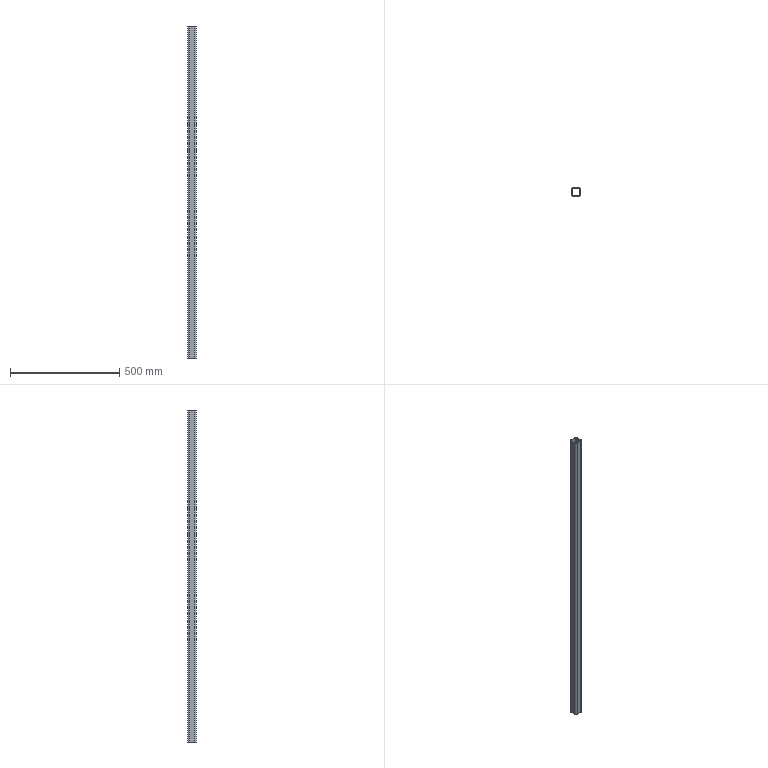Part | STEP file | 40 x 40 x 1200-2 | 1 solid | 18 faces | box 40 x 40 x 1520 mm | volume 812891 mm3 | plane 10 | cylinder 8 | commonest cylinder face diameters 8 x4 16 x4
STEP:
#1=CARTESIAN_POINT('',(32.,40.,600.));
#2=VERTEX_POINT('',#1);
#3=CARTESIAN_POINT('',(8.,40.,600.));
#4=VERTEX_POINT('',#3);
#5=CARTESIAN_POINT('',(32.,40.,600.));
#6=DIRECTION('',(-1.,0.,0.));
#7=VECTOR('',#6,1000.);
#8=LINE('',#5,#7);
#9=EDGE_CURVE('',#2,#4,#8,.T.);
#10=ORIENTED_EDGE('',*,*,#9,.F.);
#11=CARTESIAN_POINT('',(32.,40.,-920.));
#12=VERTEX_POINT('',#11);
#13=CARTESIAN_POINT('',(32.,40.,600.));
#14=DIRECTION('',(0.,0.,1.));
#15=VECTOR('',#14,1000.);
#16=LINE('',#13,#15);
#17=EDGE_CURVE('',#12,#2,#16,.T.);
#18=ORIENTED_EDGE('',*,*,#17,.F.);
#19=CARTESIAN_POINT('',(8.,40.,-920.));
#20=VERTEX_POINT('',#19);
#21=CARTESIAN_POINT('',(8.,40.,-920.));
#22=DIRECTION('',(-1.,0.,0.));
#23=VECTOR('',#22,1000.);
#24=LINE('',#21,#23);
#25=EDGE_CURVE('',#12,#20,#24,.T.);
#26=ORIENTED_EDGE('',*,*,#25,.T.);
#27=CARTESIAN_POINT('',(8.,40.,600.));
#28=DIRECTION('',(0.,0.,-1.));
#29=VECTOR('',#28,1000.);
#30=LINE('',#27,#29);
#31=EDGE_CURVE('',#4,#20,#30,.T.);
#32=ORIENTED_EDGE('',*,*,#31,.F.);
#33=EDGE_LOOP('',(#10,#18,#26,#32));
#34=FACE_OUTER_BOUND('',#33,.T.);
#35=CARTESIAN_POINT('',(32.,40.,600.));
#36=DIRECTION('',(0.,-1.,0.));
#37=DIRECTION('',(1.,0.,0.));
#38=AXIS2_PLACEMENT_3D('',#35,#36,#37);
#39=PLANE('',#38);
#40=ADVANCED_FACE('',(#34),#39,.F.);
#41=ORIENTED_EDGE('',*,*,#31,.T.);
#42=CARTESIAN_POINT('',(0.,32.,-920.));
#43=VERTEX_POINT('',#42);
#44=CARTESIAN_POINT('',(8.,32.,-920.));
#45=DIRECTION('',(0.,0.,1.));
#46=DIRECTION('',(1.,0.,0.));
#47=AXIS2_PLACEMENT_3D('',#44,#45,#46);
#48=CIRCLE('',#47,8.);
#49=EDGE_CURVE('',#20,#43,#48,.T.);
#50=ORIENTED_EDGE('',*,*,#49,.T.);
#51=CARTESIAN_POINT('',(0.,32.,600.));
#52=VERTEX_POINT('',#51);
#53=CARTESIAN_POINT('',(0.,32.,600.));
#54=DIRECTION('',(0.,0.,1.));
#55=VECTOR('',#54,1000.);
#56=LINE('',#53,#55);
#57=EDGE_CURVE('',#43,#52,#56,.T.);
#58=ORIENTED_EDGE('',*,*,#57,.T.);
#59=CARTESIAN_POINT('',(8.,32.,600.));
#60=DIRECTION('',(0.,0.,-1.));
#61=DIRECTION('',(-1.,0.,0.));
#62=AXIS2_PLACEMENT_3D('',#59,#60,#61);
#63=CIRCLE('',#62,8.);
#64=EDGE_CURVE('',#52,#4,#63,.T.);
#65=ORIENTED_EDGE('',*,*,#64,.T.);
#66=EDGE_LOOP('',(#41,#50,#58,#65));
#67=FACE_OUTER_BOUND('',#66,.T.);
#68=CARTESIAN_POINT('',(8.,32.,600.));
#69=DIRECTION('',(0.,0.,-1.));
#70=DIRECTION('',(-1.,0.,0.));
#71=AXIS2_PLACEMENT_3D('',#68,#69,#70);
#72=CYLINDRICAL_SURFACE('',#71,8.);
#73=ADVANCED_FACE('',(#67),#72,.T.);
#74=CARTESIAN_POINT('',(0.,8.,600.));
#75=VERTEX_POINT('',#74);
#76=CARTESIAN_POINT('',(8.,0.,600.));
#77=VERTEX_POINT('',#76);
#78=CARTESIAN_POINT('',(8.,8.,600.));
#79=DIRECTION('',(0.,0.,1.));
#80=DIRECTION('',(-1.,0.,0.));
#81=AXIS2_PLACEMENT_3D('',#78,#79,#80);
#82=CIRCLE('',#81,8.);
#83=EDGE_CURVE('',#75,#77,#82,.T.);
#84=ORIENTED_EDGE('',*,*,#83,.T.);
#85=CARTESIAN_POINT('',(32.,0.,600.));
#86=VERTEX_POINT('',#85);
#87=CARTESIAN_POINT('',(32.,0.,600.));
#88=DIRECTION('',(1.,0.,0.));
#89=VECTOR('',#88,1000.);
#90=LINE('',#87,#89);
#91=EDGE_CURVE('',#77,#86,#90,.T.);
#92=ORIENTED_EDGE('',*,*,#91,.T.);
#93=CARTESIAN_POINT('',(40.,8.,600.));
#94=VERTEX_POINT('',#93);
#95=CARTESIAN_POINT('',(32.,8.,600.));
#96=DIRECTION('',(0.,0.,1.));
#97=DIRECTION('',(-1.,0.,0.));
#98=AXIS2_PLACEMENT_3D('',#95,#96,#97);
#99=CIRCLE('',#98,8.);
#100=EDGE_CURVE('',#86,#94,#99,.T.);
#101=ORIENTED_EDGE('',*,*,#100,.T.);
#102=CARTESIAN_POINT('',(40.,32.,600.));
#103=VERTEX_POINT('',#102);
#104=CARTESIAN_POINT('',(40.,32.,600.));
#105=DIRECTION('',(0.,1.,0.));
#106=VECTOR('',#105,1000.);
#107=LINE('',#104,#106);
#108=EDGE_CURVE('',#94,#103,#107,.T.);
#109=ORIENTED_EDGE('',*,*,#108,.T.);
#110=CARTESIAN_POINT('',(32.,32.,600.));
#111=DIRECTION('',(0.,0.,1.));
#112=DIRECTION('',(-1.,0.,0.));
#113=AXIS2_PLACEMENT_3D('',#110,#111,#112);
#114=CIRCLE('',#113,8.);
#115=EDGE_CURVE('',#103,#2,#114,.T.);
#116=ORIENTED_EDGE('',*,*,#115,.T.);
#117=ORIENTED_EDGE('',*,*,#9,.T.);
#118=ORIENTED_EDGE('',*,*,#64,.F.);
#119=CARTESIAN_POINT('',(0.,32.,600.));
#120=DIRECTION('',(0.,-1.,0.));
#121=VECTOR('',#120,1000.);
#122=LINE('',#119,#121);
#123=EDGE_CURVE('',#52,#75,#122,.T.);
#124=ORIENTED_EDGE('',*,*,#123,.T.);
#125=EDGE_LOOP('',(#84,#92,#101,#109,#116,#117,#118,#124));
#126=FACE_OUTER_BOUND('',#125,.T.);
#127=CARTESIAN_POINT('',(36.,32.,600.));
#128=VERTEX_POINT('',#127);
#129=CARTESIAN_POINT('',(36.,8.,600.));
#130=VERTEX_POINT('',#129);
#131=CARTESIAN_POINT('',(36.,32.,600.));
#132=DIRECTION('',(0.,-1.,0.));
#133=VECTOR('',#132,1000.);
#134=LINE('',#131,#133);
#135=EDGE_CURVE('',#128,#130,#134,.T.);
#136=ORIENTED_EDGE('',*,*,#135,.T.);
#137=CARTESIAN_POINT('',(32.,4.,600.));
#138=VERTEX_POINT('',#137);
#139=CARTESIAN_POINT('',(32.,8.,600.));
#140=DIRECTION('',(0.,0.,-1.));
#141=DIRECTION('',(-1.,0.,0.));
#142=AXIS2_PLACEMENT_3D('',#139,#140,#141);
#143=CIRCLE('',#142,4.);
#144=EDGE_CURVE('',#130,#138,#143,.T.);
#145=ORIENTED_EDGE('',*,*,#144,.T.);
#146=CARTESIAN_POINT('',(8.,4.,600.));
#147=VERTEX_POINT('',#146);
#148=CARTESIAN_POINT('',(32.,4.,600.));
#149=DIRECTION('',(-1.,0.,0.));
#150=VECTOR('',#149,1000.);
#151=LINE('',#148,#150);
#152=EDGE_CURVE('',#138,#147,#151,.T.);
#153=ORIENTED_EDGE('',*,*,#152,.T.);
#154=CARTESIAN_POINT('',(4.,8.,600.));
#155=VERTEX_POINT('',#154);
#156=CARTESIAN_POINT('',(8.,8.,600.));
#157=DIRECTION('',(0.,0.,-1.));
#158=DIRECTION('',(-1.,0.,0.));
#159=AXIS2_PLACEMENT_3D('',#156,#157,#158);
#160=CIRCLE('',#159,4.);
#161=EDGE_CURVE('',#147,#155,#160,.T.);
#162=ORIENTED_EDGE('',*,*,#161,.T.);
#163=CARTESIAN_POINT('',(4.,32.,600.));
#164=VERTEX_POINT('',#163);
#165=CARTESIAN_POINT('',(4.,32.,600.));
#166=DIRECTION('',(0.,1.,0.));
#167=VECTOR('',#166,1000.);
#168=LINE('',#165,#167);
#169=EDGE_CURVE('',#155,#164,#168,.T.);
#170=ORIENTED_EDGE('',*,*,#169,.T.);
#171=CARTESIAN_POINT('',(8.,36.,600.));
#172=VERTEX_POINT('',#171);
#173=CARTESIAN_POINT('',(8.,32.,600.));
#174=DIRECTION('',(0.,0.,-1.));
#175=DIRECTION('',(-1.,0.,0.));
#176=AXIS2_PLACEMENT_3D('',#173,#174,#175);
#177=CIRCLE('',#176,4.);
#178=EDGE_CURVE('',#164,#172,#177,.T.);
#179=ORIENTED_EDGE('',*,*,#178,.T.);
#180=CARTESIAN_POINT('',(32.,36.,600.));
#181=VERTEX_POINT('',#180);
#182=CARTESIAN_POINT('',(32.,36.,600.));
#183=DIRECTION('',(1.,0.,0.));
#184=VECTOR('',#183,1000.);
#185=LINE('',#182,#184);
#186=EDGE_CURVE('',#172,#181,#185,.T.);
#187=ORIENTED_EDGE('',*,*,#186,.T.);
#188=CARTESIAN_POINT('',(32.,32.,600.));
#189=DIRECTION('',(0.,0.,-1.));
#190=DIRECTION('',(-1.,0.,0.));
#191=AXIS2_PLACEMENT_3D('',#188,#189,#190);
#192=CIRCLE('',#191,4.);
#193=EDGE_CURVE('',#181,#128,#192,.T.);
#194=ORIENTED_EDGE('',*,*,#193,.T.);
#195=EDGE_LOOP('',(#136,#145,#153,#162,#170,#179,#187,#194));
#196=FACE_BOUND('',#195,.T.);
#197=CARTESIAN_POINT('',(32.,32.,600.));
#198=DIRECTION('',(0.,0.,1.));
#199=DIRECTION('',(1.,0.,0.));
#200=AXIS2_PLACEMENT_3D('',#197,#198,#199);
#201=PLANE('',#200);
#202=ADVANCED_FACE('',(#126,#196),#201,.T.);
#203=CARTESIAN_POINT('',(40.,32.,-920.));
#204=VERTEX_POINT('',#203);
#205=CARTESIAN_POINT('',(40.,32.,600.));
#206=DIRECTION('',(0.,0.,-1.));
#207=VECTOR('',#206,1000.);
#208=LINE('',#205,#207);
#209=EDGE_CURVE('',#103,#204,#208,.T.);
#210=ORIENTED_EDGE('',*,*,#209,.T.);
#211=CARTESIAN_POINT('',(32.,32.,-920.));
#212=DIRECTION('',(0.,0.,1.));
#213=DIRECTION('',(1.,0.,0.));
#214=AXIS2_PLACEMENT_3D('',#211,#212,#213);
#215=CIRCLE('',#214,8.);
#216=EDGE_CURVE('',#204,#12,#215,.T.);
#217=ORIENTED_EDGE('',*,*,#216,.T.);
#218=ORIENTED_EDGE('',*,*,#17,.T.);
#219=ORIENTED_EDGE('',*,*,#115,.F.);
#220=EDGE_LOOP('',(#210,#217,#218,#219));
#221=FACE_OUTER_BOUND('',#220,.T.);
#222=CARTESIAN_POINT('',(32.,32.,600.));
#223=DIRECTION('',(0.,0.,-1.));
#224=DIRECTION('',(-1.,0.,0.));
#225=AXIS2_PLACEMENT_3D('',#222,#223,#224);
#226=CYLINDRICAL_SURFACE('',#225,8.);
#227=ADVANCED_FACE('',(#221),#226,.T.);
#228=ORIENTED_EDGE('',*,*,#123,.F.);
#229=ORIENTED_EDGE('',*,*,#57,.F.);
#230=CARTESIAN_POINT('',(0.,8.,-920.));
#231=VERTEX_POINT('',#230);
#232=CARTESIAN_POINT('',(0.,8.,-920.));
#233=DIRECTION('',(0.,-1.,0.));
#234=VECTOR('',#233,1000.);
#235=LINE('',#232,#234);
#236=EDGE_CURVE('',#43,#231,#235,.T.);
#237=ORIENTED_EDGE('',*,*,#236,.T.);
#238=CARTESIAN_POINT('',(0.,8.,600.));
#239=DIRECTION('',(0.,0.,-1.));
#240=VECTOR('',#239,1000.);
#241=LINE('',#238,#240);
#242=EDGE_CURVE('',#75,#231,#241,.T.);
#243=ORIENTED_EDGE('',*,*,#242,.F.);
#244=EDGE_LOOP('',(#228,#229,#237,#243));
#245=FACE_OUTER_BOUND('',#244,.T.);
#246=CARTESIAN_POINT('',(0.,8.,600.));
#247=DIRECTION('',(1.,0.,0.));
#248=DIRECTION('',(0.,1.,0.));
#249=AXIS2_PLACEMENT_3D('',#246,#247,#248);
#250=PLANE('',#249);
#251=ADVANCED_FACE('',(#245),#250,.F.);
#252=ORIENTED_EDGE('',*,*,#91,.F.);
#253=CARTESIAN_POINT('',(8.,0.,-920.));
#254=VERTEX_POINT('',#253);
#255=CARTESIAN_POINT('',(8.,0.,600.));
#256=DIRECTION('',(0.,0.,1.));
#257=VECTOR('',#256,1000.);
#258=LINE('',#255,#257);
#259=EDGE_CURVE('',#254,#77,#258,.T.);
#260=ORIENTED_EDGE('',*,*,#259,.F.);
#261=CARTESIAN_POINT('',(32.,0.,-920.));
#262=VERTEX_POINT('',#261);
#263=CARTESIAN_POINT('',(32.,0.,-920.));
#264=DIRECTION('',(1.,0.,0.));
#265=VECTOR('',#264,1000.);
#266=LINE('',#263,#265);
#267=EDGE_CURVE('',#254,#262,#266,.T.);
#268=ORIENTED_EDGE('',*,*,#267,.T.);
#269=CARTESIAN_POINT('',(32.,0.,600.));
#270=DIRECTION('',(0.,0.,-1.));
#271=VECTOR('',#270,1000.);
#272=LINE('',#269,#271);
#273=EDGE_CURVE('',#86,#262,#272,.T.);
#274=ORIENTED_EDGE('',*,*,#273,.F.);
#275=EDGE_LOOP('',(#252,#260,#268,#274));
#276=FACE_OUTER_BOUND('',#275,.T.);
#277=CARTESIAN_POINT('',(8.,0.,600.));
#278=DIRECTION('',(0.,1.,0.));
#279=DIRECTION('',(-1.,0.,0.));
#280=AXIS2_PLACEMENT_3D('',#277,#278,#279);
#281=PLANE('',#280);
#282=ADVANCED_FACE('',(#276),#281,.F.);
#283=ORIENTED_EDGE('',*,*,#242,.T.);
#284=CARTESIAN_POINT('',(8.,8.,-920.));
#285=DIRECTION('',(0.,0.,1.));
#286=DIRECTION('',(1.,0.,0.));
#287=AXIS2_PLACEMENT_3D('',#284,#285,#286);
#288=CIRCLE('',#287,8.);
#289=EDGE_CURVE('',#231,#254,#288,.T.);
#290=ORIENTED_EDGE('',*,*,#289,.T.);
#291=ORIENTED_EDGE('',*,*,#259,.T.);
#292=ORIENTED_EDGE('',*,*,#83,.F.);
#293=EDGE_LOOP('',(#283,#290,#291,#292));
#294=FACE_OUTER_BOUND('',#293,.T.);
#295=CARTESIAN_POINT('',(8.,8.,600.));
#296=DIRECTION('',(0.,0.,-1.));
#297=DIRECTION('',(-1.,0.,0.));
#298=AXIS2_PLACEMENT_3D('',#295,#296,#297);
#299=CYLINDRICAL_SURFACE('',#298,8.);
#300=ADVANCED_FACE('',(#294),#299,.T.);
#301=ORIENTED_EDGE('',*,*,#108,.F.);
#302=CARTESIAN_POINT('',(40.,8.,-920.));
#303=VERTEX_POINT('',#302);
#304=CARTESIAN_POINT('',(40.,8.,600.));
#305=DIRECTION('',(0.,0.,1.));
#306=VECTOR('',#305,1000.);
#307=LINE('',#304,#306);
#308=EDGE_CURVE('',#303,#94,#307,.T.);
#309=ORIENTED_EDGE('',*,*,#308,.F.);
#310=CARTESIAN_POINT('',(40.,32.,-920.));
#311=DIRECTION('',(0.,1.,0.));
#312=VECTOR('',#311,1000.);
#313=LINE('',#310,#312);
#314=EDGE_CURVE('',#303,#204,#313,.T.);
#315=ORIENTED_EDGE('',*,*,#314,.T.);
#316=ORIENTED_EDGE('',*,*,#209,.F.);
#317=EDGE_LOOP('',(#301,#309,#315,#316));
#318=FACE_OUTER_BOUND('',#317,.T.);
#319=CARTESIAN_POINT('',(40.,32.,600.));
#320=DIRECTION('',(-1.,0.,0.));
#321=DIRECTION('',(0.,-1.,0.));
#322=AXIS2_PLACEMENT_3D('',#319,#320,#321);
#323=PLANE('',#322);
#324=ADVANCED_FACE('',(#318),#323,.F.);
#325=ORIENTED_EDGE('',*,*,#273,.T.);
#326=CARTESIAN_POINT('',(32.,8.,-920.));
#327=DIRECTION('',(0.,0.,1.));
#328=DIRECTION('',(1.,0.,0.));
#329=AXIS2_PLACEMENT_3D('',#326,#327,#328);
#330=CIRCLE('',#329,8.);
#331=EDGE_CURVE('',#262,#303,#330,.T.);
#332=ORIENTED_EDGE('',*,*,#331,.T.);
#333=ORIENTED_EDGE('',*,*,#308,.T.);
#334=ORIENTED_EDGE('',*,*,#100,.F.);
#335=EDGE_LOOP('',(#325,#332,#333,#334));
#336=FACE_OUTER_BOUND('',#335,.T.);
#337=CARTESIAN_POINT('',(32.,8.,600.));
#338=DIRECTION('',(0.,0.,-1.));
#339=DIRECTION('',(-1.,0.,0.));
#340=AXIS2_PLACEMENT_3D('',#337,#338,#339);
#341=CYLINDRICAL_SURFACE('',#340,8.);
#342=ADVANCED_FACE('',(#336),#341,.T.);
#343=ORIENTED_EDGE('',*,*,#144,.F.);
#344=CARTESIAN_POINT('',(36.,8.,-920.));
#345=VERTEX_POINT('',#344);
#346=CARTESIAN_POINT('',(36.,8.,600.));
#347=DIRECTION('',(0.,0.,1.));
#348=VECTOR('',#347,1000.);
#349=LINE('',#346,#348);
#350=EDGE_CURVE('',#345,#130,#349,.T.);
#351=ORIENTED_EDGE('',*,*,#350,.F.);
#352=CARTESIAN_POINT('',(32.,4.,-920.));
#353=VERTEX_POINT('',#352);
#354=CARTESIAN_POINT('',(32.,8.,-920.));
#355=DIRECTION('',(0.,0.,1.));
#356=DIRECTION('',(1.,0.,0.));
#357=AXIS2_PLACEMENT_3D('',#354,#355,#356);
#358=CIRCLE('',#357,4.);
#359=EDGE_CURVE('',#353,#345,#358,.T.);
#360=ORIENTED_EDGE('',*,*,#359,.F.);
#361=CARTESIAN_POINT('',(32.,4.,600.));
#362=DIRECTION('',(0.,0.,-1.));
#363=VECTOR('',#362,1000.);
#364=LINE('',#361,#363);
#365=EDGE_CURVE('',#138,#353,#364,.T.);
#366=ORIENTED_EDGE('',*,*,#365,.F.);
#367=EDGE_LOOP('',(#343,#351,#360,#366));
#368=FACE_OUTER_BOUND('',#367,.T.);
#369=CARTESIAN_POINT('',(32.,8.,600.));
#370=DIRECTION('',(0.,0.,-1.));
#371=DIRECTION('',(-1.,0.,0.));
#372=AXIS2_PLACEMENT_3D('',#369,#370,#371);
#373=CYLINDRICAL_SURFACE('',#372,4.);
#374=ADVANCED_FACE('',(#368),#373,.F.);
#375=CARTESIAN_POINT('',(36.,32.,-920.));
#376=VERTEX_POINT('',#375);
#377=CARTESIAN_POINT('',(36.,32.,600.));
#378=DIRECTION('',(0.,0.,-1.));
#379=VECTOR('',#378,1000.);
#380=LINE('',#377,#379);
#381=EDGE_CURVE('',#128,#376,#380,.T.);
#382=ORIENTED_EDGE('',*,*,#381,.T.);
#383=CARTESIAN_POINT('',(36.,32.,-920.));
#384=DIRECTION('',(0.,1.,0.));
#385=VECTOR('',#384,1000.);
#386=LINE('',#383,#385);
#387=EDGE_CURVE('',#345,#376,#386,.T.);
#388=ORIENTED_EDGE('',*,*,#387,.F.);
#389=ORIENTED_EDGE('',*,*,#350,.T.);
#390=ORIENTED_EDGE('',*,*,#135,.F.);
#391=EDGE_LOOP('',(#382,#388,#389,#390));
#392=FACE_OUTER_BOUND('',#391,.T.);
#393=CARTESIAN_POINT('',(36.,32.,600.));
#394=DIRECTION('',(-1.,0.,0.));
#395=DIRECTION('',(0.,0.,1.));
#396=AXIS2_PLACEMENT_3D('',#393,#394,#395);
#397=PLANE('',#396);
#398=ADVANCED_FACE('',(#392),#397,.T.);
#399=ORIENTED_EDGE('',*,*,#193,.F.);
#400=CARTESIAN_POINT('',(32.,36.,-920.));
#401=VERTEX_POINT('',#400);
#402=CARTESIAN_POINT('',(32.,36.,600.));
#403=DIRECTION('',(0.,0.,1.));
#404=VECTOR('',#403,1000.);
#405=LINE('',#402,#404);
#406=EDGE_CURVE('',#401,#181,#405,.T.);
#407=ORIENTED_EDGE('',*,*,#406,.F.);
#408=CARTESIAN_POINT('',(32.,32.,-920.));
#409=DIRECTION('',(0.,0.,1.));
#410=DIRECTION('',(1.,0.,0.));
#411=AXIS2_PLACEMENT_3D('',#408,#409,#410);
#412=CIRCLE('',#411,4.);
#413=EDGE_CURVE('',#376,#401,#412,.T.);
#414=ORIENTED_EDGE('',*,*,#413,.F.);
#415=ORIENTED_EDGE('',*,*,#381,.F.);
#416=EDGE_LOOP('',(#399,#407,#414,#415));
#417=FACE_OUTER_BOUND('',#416,.T.);
#418=CARTESIAN_POINT('',(32.,32.,600.));
#419=DIRECTION('',(0.,0.,-1.));
#420=DIRECTION('',(-1.,0.,0.));
#421=AXIS2_PLACEMENT_3D('',#418,#419,#420);
#422=CYLINDRICAL_SURFACE('',#421,4.);
#423=ADVANCED_FACE('',(#417),#422,.F.);
#424=CARTESIAN_POINT('',(8.,36.,-920.));
#425=VERTEX_POINT('',#424);
#426=CARTESIAN_POINT('',(8.,36.,600.));
#427=DIRECTION('',(0.,0.,-1.));
#428=VECTOR('',#427,1000.);
#429=LINE('',#426,#428);
#430=EDGE_CURVE('',#172,#425,#429,.T.);
#431=ORIENTED_EDGE('',*,*,#430,.T.);
#432=CARTESIAN_POINT('',(8.,36.,-920.));
#433=DIRECTION('',(-1.,0.,0.));
#434=VECTOR('',#433,1000.);
#435=LINE('',#432,#434);
#436=EDGE_CURVE('',#401,#425,#435,.T.);
#437=ORIENTED_EDGE('',*,*,#436,.F.);
#438=ORIENTED_EDGE('',*,*,#406,.T.);
#439=ORIENTED_EDGE('',*,*,#186,.F.);
#440=EDGE_LOOP('',(#431,#437,#438,#439));
#441=FACE_OUTER_BOUND('',#440,.T.);
#442=CARTESIAN_POINT('',(32.,36.,600.));
#443=DIRECTION('',(0.,-1.,0.));
#444=DIRECTION('',(0.,0.,-1.));
#445=AXIS2_PLACEMENT_3D('',#442,#443,#444);
#446=PLANE('',#445);
#447=ADVANCED_FACE('',(#441),#446,.T.);
#448=ORIENTED_EDGE('',*,*,#178,.F.);
#449=CARTESIAN_POINT('',(4.,32.,-920.));
#450=VERTEX_POINT('',#449);
#451=CARTESIAN_POINT('',(4.,32.,600.));
#452=DIRECTION('',(0.,0.,1.));
#453=VECTOR('',#452,1000.);
#454=LINE('',#451,#453);
#455=EDGE_CURVE('',#450,#164,#454,.T.);
#456=ORIENTED_EDGE('',*,*,#455,.F.);
#457=CARTESIAN_POINT('',(8.,32.,-920.));
#458=DIRECTION('',(0.,0.,1.));
#459=DIRECTION('',(1.,0.,0.));
#460=AXIS2_PLACEMENT_3D('',#457,#458,#459);
#461=CIRCLE('',#460,4.);
#462=EDGE_CURVE('',#425,#450,#461,.T.);
#463=ORIENTED_EDGE('',*,*,#462,.F.);
#464=ORIENTED_EDGE('',*,*,#430,.F.);
#465=EDGE_LOOP('',(#448,#456,#463,#464));
#466=FACE_OUTER_BOUND('',#465,.T.);
#467=CARTESIAN_POINT('',(8.,32.,600.));
#468=DIRECTION('',(0.,0.,-1.));
#469=DIRECTION('',(-1.,0.,0.));
#470=AXIS2_PLACEMENT_3D('',#467,#468,#469);
#471=CYLINDRICAL_SURFACE('',#470,4.);
#472=ADVANCED_FACE('',(#466),#471,.F.);
#473=CARTESIAN_POINT('',(4.,8.,-920.));
#474=VERTEX_POINT('',#473);
#475=CARTESIAN_POINT('',(4.,8.,600.));
#476=DIRECTION('',(0.,0.,-1.));
#477=VECTOR('',#476,1000.);
#478=LINE('',#475,#477);
#479=EDGE_CURVE('',#155,#474,#478,.T.);
#480=ORIENTED_EDGE('',*,*,#479,.T.);
#481=CARTESIAN_POINT('',(4.,8.,-920.));
#482=DIRECTION('',(0.,-1.,0.));
#483=VECTOR('',#482,1000.);
#484=LINE('',#481,#483);
#485=EDGE_CURVE('',#450,#474,#484,.T.);
#486=ORIENTED_EDGE('',*,*,#485,.F.);
#487=ORIENTED_EDGE('',*,*,#455,.T.);
#488=ORIENTED_EDGE('',*,*,#169,.F.);
#489=EDGE_LOOP('',(#480,#486,#487,#488));
#490=FACE_OUTER_BOUND('',#489,.T.);
#491=CARTESIAN_POINT('',(4.,8.,600.));
#492=DIRECTION('',(1.,0.,0.));
#493=DIRECTION('',(0.,1.,0.));
#494=AXIS2_PLACEMENT_3D('',#491,#492,#493);
#495=PLANE('',#494);
#496=ADVANCED_FACE('',(#490),#495,.T.);
#497=ORIENTED_EDGE('',*,*,#161,.F.);
#498=CARTESIAN_POINT('',(8.,4.,-920.));
#499=VERTEX_POINT('',#498);
#500=CARTESIAN_POINT('',(8.,4.,600.));
#501=DIRECTION('',(0.,0.,1.));
#502=VECTOR('',#501,1000.);
#503=LINE('',#500,#502);
#504=EDGE_CURVE('',#499,#147,#503,.T.);
#505=ORIENTED_EDGE('',*,*,#504,.F.);
#506=CARTESIAN_POINT('',(8.,8.,-920.));
#507=DIRECTION('',(0.,0.,1.));
#508=DIRECTION('',(1.,0.,0.));
#509=AXIS2_PLACEMENT_3D('',#506,#507,#508);
#510=CIRCLE('',#509,4.);
#511=EDGE_CURVE('',#474,#499,#510,.T.);
#512=ORIENTED_EDGE('',*,*,#511,.F.);
#513=ORIENTED_EDGE('',*,*,#479,.F.);
#514=EDGE_LOOP('',(#497,#505,#512,#513));
#515=FACE_OUTER_BOUND('',#514,.T.);
#516=CARTESIAN_POINT('',(8.,8.,600.));
#517=DIRECTION('',(0.,0.,-1.));
#518=DIRECTION('',(-1.,0.,0.));
#519=AXIS2_PLACEMENT_3D('',#516,#517,#518);
#520=CYLINDRICAL_SURFACE('',#519,4.);
#521=ADVANCED_FACE('',(#515),#520,.F.);
#522=ORIENTED_EDGE('',*,*,#365,.T.);
#523=CARTESIAN_POINT('',(32.,4.,-920.));
#524=DIRECTION('',(1.,0.,0.));
#525=VECTOR('',#524,1000.);
#526=LINE('',#523,#525);
#527=EDGE_CURVE('',#499,#353,#526,.T.);
#528=ORIENTED_EDGE('',*,*,#527,.F.);
#529=ORIENTED_EDGE('',*,*,#504,.T.);
#530=ORIENTED_EDGE('',*,*,#152,.F.);
#531=EDGE_LOOP('',(#522,#528,#529,#530));
#532=FACE_OUTER_BOUND('',#531,.T.);
#533=CARTESIAN_POINT('',(8.,4.,600.));
#534=DIRECTION('',(0.,1.,0.));
#535=DIRECTION('',(-1.,0.,0.));
#536=AXIS2_PLACEMENT_3D('',#533,#534,#535);
#537=PLANE('',#536);
#538=ADVANCED_FACE('',(#532),#537,.T.);
#539=ORIENTED_EDGE('',*,*,#511,.T.);
#540=ORIENTED_EDGE('',*,*,#527,.T.);
#541=ORIENTED_EDGE('',*,*,#359,.T.);
#542=ORIENTED_EDGE('',*,*,#387,.T.);
#543=ORIENTED_EDGE('',*,*,#413,.T.);
#544=ORIENTED_EDGE('',*,*,#436,.T.);
#545=ORIENTED_EDGE('',*,*,#462,.T.);
#546=ORIENTED_EDGE('',*,*,#485,.T.);
#547=EDGE_LOOP('',(#539,#540,#541,#542,#543,#544,#545,#546));
#548=FACE_BOUND('',#547,.T.);
#549=ORIENTED_EDGE('',*,*,#267,.F.);
#550=ORIENTED_EDGE('',*,*,#289,.F.);
#551=ORIENTED_EDGE('',*,*,#236,.F.);
#552=ORIENTED_EDGE('',*,*,#49,.F.);
#553=ORIENTED_EDGE('',*,*,#25,.F.);
#554=ORIENTED_EDGE('',*,*,#216,.F.);
#555=ORIENTED_EDGE('',*,*,#314,.F.);
#556=ORIENTED_EDGE('',*,*,#331,.F.);
#557=EDGE_LOOP('',(#549,#550,#551,#552,#553,#554,#555,#556));
#558=FACE_OUTER_BOUND('',#557,.T.);
#559=CARTESIAN_POINT('',(-1640.,-56.,-920.));
#560=DIRECTION('',(0.,0.,1.));
#561=DIRECTION('',(0.,1.,0.));
#562=AXIS2_PLACEMENT_3D('',#559,#560,#561);
#563=PLANE('',#562);
#564=ADVANCED_FACE('',(#548,#558),#563,.F.);
#565=CLOSED_SHELL('',(#40,#73,#202,#227,#251,#282,#300,#324,#342,#374,#398,#423,#447,#472,#496,#521,#538,#564));
#566=MANIFOLD_SOLID_BREP('',#565);
#567=CARTESIAN_POINT('',(0.,0.,0.));
#568=DIRECTION('',(0.,0.,1.));
#569=DIRECTION('',(1.,0.,0.));
#570=AXIS2_PLACEMENT_3D('',#567,#568,#569);
#571=(LENGTH_UNIT()NAMED_UNIT(*)SI_UNIT(.MILLI.,.METRE.));
#572=UNCERTAINTY_MEASURE_WITH_UNIT(LENGTH_MEASURE(0.00001),#571,'','');
#573=(NAMED_UNIT(*)PLANE_ANGLE_UNIT()SI_UNIT($,.RADIAN.));
#574=(NAMED_UNIT(*)SI_UNIT($,.STERADIAN.)SOLID_ANGLE_UNIT());
#575=(GEOMETRIC_REPRESENTATION_CONTEXT(3)GLOBAL_UNCERTAINTY_ASSIGNED_CONTEXT((#572))GLOBAL_UNIT_ASSIGNED_CONTEXT((#571,#573,#574))REPRESENTATION_CONTEXT('',''));
#576=ADVANCED_BREP_SHAPE_REPRESENTATION('',(#566,#570),#575);